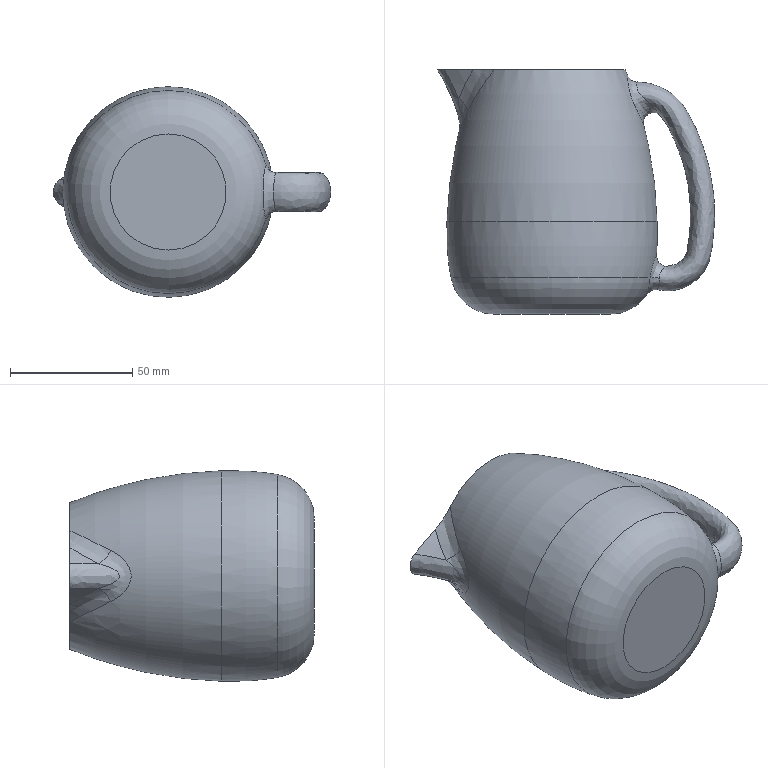Part | NX | features DATUM_CSYS 3, REPLACE_FACE 3, SKETCH 3, BLEND 2, OFFSET_REGION 2, SKIN 2, UNITE 2, DATUM_ON_PATH 1, SHELL 1, SWP104 1 | 1 solid | 25 faces | box 113.54 x 100 x 86.236 mm | volume 41755 mm3 | spline 16 | torus 6 | plane 3